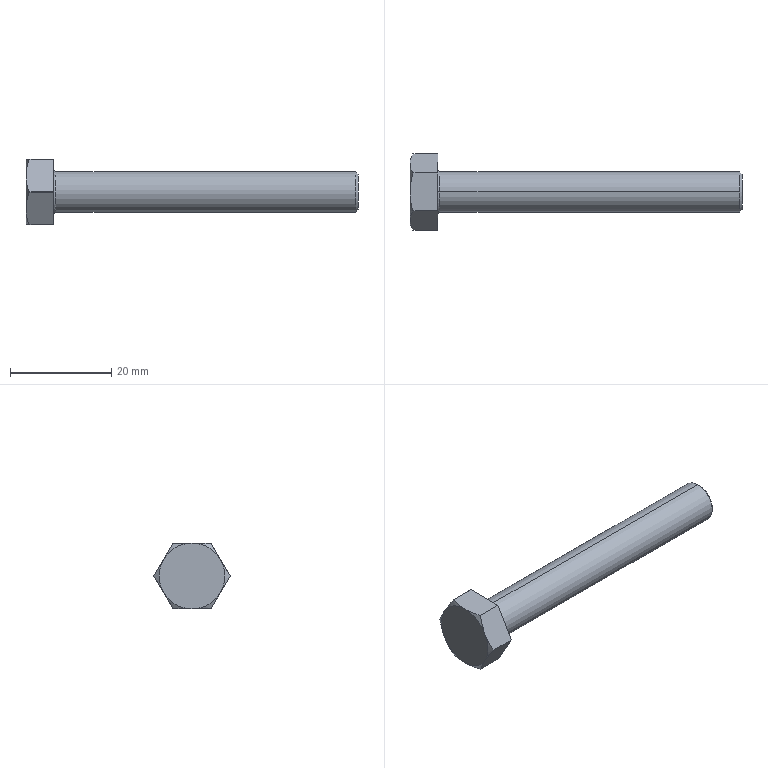Part | NX | features STRCB8-60 2 | 1 solid | 27 faces | box 65.5 x 15 x 13 mm | volume 3817 mm3 | plane 9 | cone 8 | cylinder 8 | torus 2 | commonest cylinder face diameters 15 x6 8 x2
STEP:
#1=CARTESIAN_POINT('',(145.215,66.,-9.5));
#2=VERTEX_POINT('',#1);
#3=CARTESIAN_POINT('',(145.215,60.371,-6.25));
#4=VERTEX_POINT('',#3);
#5=CARTESIAN_POINT('',(145.215,66.,-3.));
#6=DIRECTION('',(-1.,0.,0.));
#7=DIRECTION('',(0.,0.,-1.));
#8=AXIS2_PLACEMENT_3D('',#5,#6,#7);
#9=CIRCLE('',#8,6.5);
#10=EDGE_CURVE('',#2,#4,#9,.T.);
#11=ORIENTED_EDGE('',*,*,#10,.F.);
#12=CARTESIAN_POINT('',(145.793,62.258,-9.5));
#13=VERTEX_POINT('',#12);
#14=CARTESIAN_POINT('',(145.215,66.,-9.5));
#15=CARTESIAN_POINT('',(145.214,64.733,-9.5));
#16=CARTESIAN_POINT('',(145.442,63.474,-9.5));
#17=CARTESIAN_POINT('',(145.793,62.258,-9.5));
#18=B_SPLINE_CURVE_WITH_KNOTS('',3,(#14,#15,#16,#17),.UNSPECIFIED.,.F.,.F.,(4,4),(0.,1.),.UNSPECIFIED.);
#19=EDGE_CURVE('',#2,#13,#18,.T.);
#20=ORIENTED_EDGE('',*,*,#19,.T.);
#21=CARTESIAN_POINT('',(145.793,62.242,-9.49));
#22=VERTEX_POINT('',#21);
#23=CARTESIAN_POINT('',(145.793,66.,-3.));
#24=DIRECTION('',(-1.,0.,0.));
#25=DIRECTION('',(0.,-0.4989,-0.8667));
#26=AXIS2_PLACEMENT_3D('',#23,#24,#25);
#27=CIRCLE('',#26,7.5);
#28=EDGE_CURVE('',#13,#22,#27,.T.);
#29=ORIENTED_EDGE('',*,*,#28,.T.);
#30=CARTESIAN_POINT('',(145.793,62.242,-9.49));
#31=CARTESIAN_POINT('',(145.442,61.634,-8.437));
#32=CARTESIAN_POINT('',(145.214,61.004,-7.347));
#33=CARTESIAN_POINT('',(145.215,60.371,-6.25));
#34=B_SPLINE_CURVE_WITH_KNOTS('',3,(#30,#31,#32,#33),.UNSPECIFIED.,.F.,.F.,(4,4),(0.,1.),.UNSPECIFIED.);
#35=EDGE_CURVE('',#22,#4,#34,.T.);
#36=ORIENTED_EDGE('',*,*,#35,.T.);
#37=EDGE_LOOP('',(#11,#20,#29,#36));
#38=FACE_BOUND('',#37,.T.);
#39=CARTESIAN_POINT('',(145.174,66.,-3.));
#40=DIRECTION('',(1.,0.,0.));
#41=DIRECTION('',(0.,0.,1.));
#42=AXIS2_PLACEMENT_3D('',#39,#40,#41);
#43=CONICAL_SURFACE('',#42,6.428,1.047);
#44=ADVANCED_FACE('',(#38),#43,.T.);
#45=CARTESIAN_POINT('',(145.793,58.5,-3.01));
#46=VERTEX_POINT('',#45);
#47=CARTESIAN_POINT('',(145.793,58.5,-2.99));
#48=VERTEX_POINT('',#47);
#49=CARTESIAN_POINT('',(145.793,66.,-3.));
#50=DIRECTION('',(-1.,0.,0.));
#51=DIRECTION('',(0.,-1.,-0.001284));
#52=AXIS2_PLACEMENT_3D('',#49,#50,#51);
#53=CIRCLE('',#52,7.5);
#54=EDGE_CURVE('',#46,#48,#53,.T.);
#55=ORIENTED_EDGE('',*,*,#54,.T.);
#56=CARTESIAN_POINT('',(145.215,60.371,0.25));
#57=VERTEX_POINT('',#56);
#58=CARTESIAN_POINT('',(145.793,58.5,-2.99));
#59=CARTESIAN_POINT('',(145.442,59.108,-1.937));
#60=CARTESIAN_POINT('',(145.214,59.737,-0.847));
#61=CARTESIAN_POINT('',(145.215,60.371,0.25));
#62=B_SPLINE_CURVE_WITH_KNOTS('',3,(#58,#59,#60,#61),.UNSPECIFIED.,.F.,.F.,(4,4),(0.,1.),.UNSPECIFIED.);
#63=EDGE_CURVE('',#48,#57,#62,.T.);
#64=ORIENTED_EDGE('',*,*,#63,.T.);
#65=CARTESIAN_POINT('',(145.215,66.,-3.));
#66=DIRECTION('',(-1.,0.,0.));
#67=DIRECTION('',(0.,-0.866,-0.5));
#68=AXIS2_PLACEMENT_3D('',#65,#66,#67);
#69=CIRCLE('',#68,6.5);
#70=EDGE_CURVE('',#4,#57,#69,.T.);
#71=ORIENTED_EDGE('',*,*,#70,.F.);
#72=CARTESIAN_POINT('',(145.215,60.371,-6.25));
#73=CARTESIAN_POINT('',(145.214,59.737,-5.153));
#74=CARTESIAN_POINT('',(145.442,59.108,-4.063));
#75=CARTESIAN_POINT('',(145.793,58.5,-3.01));
#76=B_SPLINE_CURVE_WITH_KNOTS('',3,(#72,#73,#74,#75),.UNSPECIFIED.,.F.,.F.,(4,4),(0.,1.),.UNSPECIFIED.);
#77=EDGE_CURVE('',#4,#46,#76,.T.);
#78=ORIENTED_EDGE('',*,*,#77,.T.);
#79=EDGE_LOOP('',(#55,#64,#71,#78));
#80=FACE_BOUND('',#79,.T.);
#81=CARTESIAN_POINT('',(145.174,66.,-3.));
#82=DIRECTION('',(1.,0.,0.));
#83=DIRECTION('',(0.,0.,1.));
#84=AXIS2_PLACEMENT_3D('',#81,#82,#83);
#85=CONICAL_SURFACE('',#84,6.428,1.047);
#86=ADVANCED_FACE('',(#80),#85,.T.);
#87=CARTESIAN_POINT('',(145.215,66.,3.5));
#88=VERTEX_POINT('',#87);
#89=CARTESIAN_POINT('',(145.215,66.,-3.));
#90=DIRECTION('',(-1.,0.,0.));
#91=DIRECTION('',(0.,-0.866,0.5));
#92=AXIS2_PLACEMENT_3D('',#89,#90,#91);
#93=CIRCLE('',#92,6.5);
#94=EDGE_CURVE('',#57,#88,#93,.T.);
#95=ORIENTED_EDGE('',*,*,#94,.F.);
#96=CARTESIAN_POINT('',(145.793,62.242,3.49));
#97=VERTEX_POINT('',#96);
#98=CARTESIAN_POINT('',(145.215,60.371,0.25));
#99=CARTESIAN_POINT('',(145.214,61.004,1.347));
#100=CARTESIAN_POINT('',(145.442,61.634,2.437));
#101=CARTESIAN_POINT('',(145.793,62.242,3.49));
#102=B_SPLINE_CURVE_WITH_KNOTS('',3,(#98,#99,#100,#101),.UNSPECIFIED.,.F.,.F.,(4,4),(0.,1.),.UNSPECIFIED.);
#103=EDGE_CURVE('',#57,#97,#102,.T.);
#104=ORIENTED_EDGE('',*,*,#103,.T.);
#105=CARTESIAN_POINT('',(145.793,62.258,3.5));
#106=VERTEX_POINT('',#105);
#107=CARTESIAN_POINT('',(145.793,66.,-3.));
#108=DIRECTION('',(-1.,0.,0.));
#109=DIRECTION('',(0.,-0.5011,0.8654));
#110=AXIS2_PLACEMENT_3D('',#107,#108,#109);
#111=CIRCLE('',#110,7.5);
#112=EDGE_CURVE('',#97,#106,#111,.T.);
#113=ORIENTED_EDGE('',*,*,#112,.T.);
#114=CARTESIAN_POINT('',(145.793,62.258,3.5));
#115=CARTESIAN_POINT('',(145.442,63.474,3.5));
#116=CARTESIAN_POINT('',(145.214,64.733,3.5));
#117=CARTESIAN_POINT('',(145.215,66.,3.5));
#118=B_SPLINE_CURVE_WITH_KNOTS('',3,(#114,#115,#116,#117),.UNSPECIFIED.,.F.,.F.,(4,4),(0.,1.),.UNSPECIFIED.);
#119=EDGE_CURVE('',#106,#88,#118,.T.);
#120=ORIENTED_EDGE('',*,*,#119,.T.);
#121=EDGE_LOOP('',(#95,#104,#113,#120));
#122=FACE_BOUND('',#121,.T.);
#123=CARTESIAN_POINT('',(145.174,66.,-3.));
#124=DIRECTION('',(1.,0.,0.));
#125=DIRECTION('',(0.,0.,1.));
#126=AXIS2_PLACEMENT_3D('',#123,#124,#125);
#127=CONICAL_SURFACE('',#126,6.428,1.047);
#128=ADVANCED_FACE('',(#122),#127,.T.);
#129=CARTESIAN_POINT('',(145.793,73.5,-2.99));
#130=VERTEX_POINT('',#129);
#131=CARTESIAN_POINT('',(145.793,73.5,-3.01));
#132=VERTEX_POINT('',#131);
#133=CARTESIAN_POINT('',(145.793,66.,-3.));
#134=DIRECTION('',(-1.,0.,0.));
#135=DIRECTION('',(0.,1.,0.001284));
#136=AXIS2_PLACEMENT_3D('',#133,#134,#135);
#137=CIRCLE('',#136,7.5);
#138=EDGE_CURVE('',#130,#132,#137,.T.);
#139=ORIENTED_EDGE('',*,*,#138,.T.);
#140=CARTESIAN_POINT('',(145.215,71.629,-6.25));
#141=VERTEX_POINT('',#140);
#142=CARTESIAN_POINT('',(145.793,73.5,-3.01));
#143=CARTESIAN_POINT('',(145.442,72.892,-4.063));
#144=CARTESIAN_POINT('',(145.214,72.263,-5.153));
#145=CARTESIAN_POINT('',(145.215,71.629,-6.25));
#146=B_SPLINE_CURVE_WITH_KNOTS('',3,(#142,#143,#144,#145),.UNSPECIFIED.,.F.,.F.,(4,4),(0.,1.),.UNSPECIFIED.);
#147=EDGE_CURVE('',#132,#141,#146,.T.);
#148=ORIENTED_EDGE('',*,*,#147,.T.);
#149=CARTESIAN_POINT('',(145.215,71.629,0.25));
#150=VERTEX_POINT('',#149);
#151=CARTESIAN_POINT('',(145.215,66.,-3.));
#152=DIRECTION('',(-1.,0.,0.));
#153=DIRECTION('',(0.,0.866,0.5));
#154=AXIS2_PLACEMENT_3D('',#151,#152,#153);
#155=CIRCLE('',#154,6.5);
#156=EDGE_CURVE('',#150,#141,#155,.T.);
#157=ORIENTED_EDGE('',*,*,#156,.F.);
#158=CARTESIAN_POINT('',(145.215,71.629,0.25));
#159=CARTESIAN_POINT('',(145.214,72.263,-0.847));
#160=CARTESIAN_POINT('',(145.442,72.892,-1.937));
#161=CARTESIAN_POINT('',(145.793,73.5,-2.99));
#162=B_SPLINE_CURVE_WITH_KNOTS('',3,(#158,#159,#160,#161),.UNSPECIFIED.,.F.,.F.,(4,4),(0.,1.),.UNSPECIFIED.);
#163=EDGE_CURVE('',#150,#130,#162,.T.);
#164=ORIENTED_EDGE('',*,*,#163,.T.);
#165=EDGE_LOOP('',(#139,#148,#157,#164));
#166=FACE_BOUND('',#165,.T.);
#167=CARTESIAN_POINT('',(145.174,66.,-3.));
#168=DIRECTION('',(1.,0.,0.));
#169=DIRECTION('',(0.,0.,1.));
#170=AXIS2_PLACEMENT_3D('',#167,#168,#169);
#171=CONICAL_SURFACE('',#170,6.428,1.047);
#172=ADVANCED_FACE('',(#166),#171,.T.);
#173=CARTESIAN_POINT('',(145.215,66.,-3.));
#174=DIRECTION('',(-1.,0.,0.));
#175=DIRECTION('',(0.,0.866,-0.5));
#176=AXIS2_PLACEMENT_3D('',#173,#174,#175);
#177=CIRCLE('',#176,6.5);
#178=EDGE_CURVE('',#141,#2,#177,.T.);
#179=ORIENTED_EDGE('',*,*,#178,.F.);
#180=CARTESIAN_POINT('',(145.793,69.758,-9.49));
#181=VERTEX_POINT('',#180);
#182=CARTESIAN_POINT('',(145.215,71.629,-6.25));
#183=CARTESIAN_POINT('',(145.214,70.996,-7.347));
#184=CARTESIAN_POINT('',(145.442,70.366,-8.437));
#185=CARTESIAN_POINT('',(145.793,69.758,-9.49));
#186=B_SPLINE_CURVE_WITH_KNOTS('',3,(#182,#183,#184,#185),.UNSPECIFIED.,.F.,.F.,(4,4),(0.,1.),.UNSPECIFIED.);
#187=EDGE_CURVE('',#141,#181,#186,.T.);
#188=ORIENTED_EDGE('',*,*,#187,.T.);
#189=CARTESIAN_POINT('',(145.793,69.742,-9.5));
#190=VERTEX_POINT('',#189);
#191=CARTESIAN_POINT('',(145.793,66.,-3.));
#192=DIRECTION('',(-1.,0.,0.));
#193=DIRECTION('',(0.,0.5011,-0.8654));
#194=AXIS2_PLACEMENT_3D('',#191,#192,#193);
#195=CIRCLE('',#194,7.5);
#196=EDGE_CURVE('',#181,#190,#195,.T.);
#197=ORIENTED_EDGE('',*,*,#196,.T.);
#198=CARTESIAN_POINT('',(145.793,69.742,-9.5));
#199=CARTESIAN_POINT('',(145.442,68.526,-9.5));
#200=CARTESIAN_POINT('',(145.214,67.267,-9.5));
#201=CARTESIAN_POINT('',(145.215,66.,-9.5));
#202=B_SPLINE_CURVE_WITH_KNOTS('',3,(#198,#199,#200,#201),.UNSPECIFIED.,.F.,.F.,(4,4),(0.,1.),.UNSPECIFIED.);
#203=EDGE_CURVE('',#190,#2,#202,.T.);
#204=ORIENTED_EDGE('',*,*,#203,.T.);
#205=EDGE_LOOP('',(#179,#188,#197,#204));
#206=FACE_BOUND('',#205,.T.);
#207=CARTESIAN_POINT('',(145.174,66.,-3.));
#208=DIRECTION('',(1.,0.,0.));
#209=DIRECTION('',(0.,0.,1.));
#210=AXIS2_PLACEMENT_3D('',#207,#208,#209);
#211=CONICAL_SURFACE('',#210,6.428,1.047);
#212=ADVANCED_FACE('',(#206),#211,.T.);
#213=ORIENTED_EDGE('',*,*,#10,.T.);
#214=ORIENTED_EDGE('',*,*,#70,.T.);
#215=ORIENTED_EDGE('',*,*,#94,.T.);
#216=CARTESIAN_POINT('',(145.215,66.,-3.));
#217=DIRECTION('',(-1.,0.,0.));
#218=DIRECTION('',(0.,0.,1.));
#219=AXIS2_PLACEMENT_3D('',#216,#217,#218);
#220=CIRCLE('',#219,6.5);
#221=EDGE_CURVE('',#88,#150,#220,.T.);
#222=ORIENTED_EDGE('',*,*,#221,.T.);
#223=ORIENTED_EDGE('',*,*,#156,.T.);
#224=ORIENTED_EDGE('',*,*,#178,.T.);
#225=EDGE_LOOP('',(#213,#214,#215,#222,#223,#224));
#226=FACE_BOUND('',#225,.T.);
#227=CARTESIAN_POINT('',(145.215,62.75,-3.));
#228=DIRECTION('',(-1.,0.,0.));
#229=DIRECTION('',(0.,0.,-1.));
#230=AXIS2_PLACEMENT_3D('',#227,#228,#229);
#231=PLANE('',#230);
#232=ADVANCED_FACE('',(#226),#231,.T.);
#233=ORIENTED_EDGE('',*,*,#221,.F.);
#234=CARTESIAN_POINT('',(145.793,69.742,3.5));
#235=VERTEX_POINT('',#234);
#236=CARTESIAN_POINT('',(145.215,66.,3.5));
#237=CARTESIAN_POINT('',(145.214,67.267,3.5));
#238=CARTESIAN_POINT('',(145.442,68.526,3.5));
#239=CARTESIAN_POINT('',(145.793,69.742,3.5));
#240=B_SPLINE_CURVE_WITH_KNOTS('',3,(#236,#237,#238,#239),.UNSPECIFIED.,.F.,.F.,(4,4),(0.,1.),.UNSPECIFIED.);
#241=EDGE_CURVE('',#88,#235,#240,.T.);
#242=ORIENTED_EDGE('',*,*,#241,.T.);
#243=CARTESIAN_POINT('',(145.793,69.758,3.49));
#244=VERTEX_POINT('',#243);
#245=CARTESIAN_POINT('',(145.793,66.,-3.));
#246=DIRECTION('',(-1.,0.,0.));
#247=DIRECTION('',(0.,0.4989,0.8667));
#248=AXIS2_PLACEMENT_3D('',#245,#246,#247);
#249=CIRCLE('',#248,7.5);
#250=EDGE_CURVE('',#235,#244,#249,.T.);
#251=ORIENTED_EDGE('',*,*,#250,.T.);
#252=CARTESIAN_POINT('',(145.793,69.758,3.49));
#253=CARTESIAN_POINT('',(145.442,70.366,2.437));
#254=CARTESIAN_POINT('',(145.214,70.996,1.347));
#255=CARTESIAN_POINT('',(145.215,71.629,0.25));
#256=B_SPLINE_CURVE_WITH_KNOTS('',3,(#252,#253,#254,#255),.UNSPECIFIED.,.F.,.F.,(4,4),(0.,1.),.UNSPECIFIED.);
#257=EDGE_CURVE('',#244,#150,#256,.T.);
#258=ORIENTED_EDGE('',*,*,#257,.T.);
#259=EDGE_LOOP('',(#233,#242,#251,#258));
#260=FACE_BOUND('',#259,.T.);
#261=CARTESIAN_POINT('',(145.174,66.,-3.));
#262=DIRECTION('',(1.,0.,0.));
#263=DIRECTION('',(0.,0.,1.));
#264=AXIS2_PLACEMENT_3D('',#261,#262,#263);
#265=CONICAL_SURFACE('',#264,6.428,1.047);
#266=ADVANCED_FACE('',(#260),#265,.T.);
#267=ORIENTED_EDGE('',*,*,#250,.F.);
#268=CARTESIAN_POINT('',(150.715,69.742,3.5));
#269=VERTEX_POINT('',#268);
#270=CARTESIAN_POINT('',(145.793,69.742,3.5));
#271=DIRECTION('',(1.,0.,0.));
#272=VECTOR('',#271,1000.);
#273=LINE('',#270,#272);
#274=EDGE_CURVE('',#235,#269,#273,.T.);
#275=ORIENTED_EDGE('',*,*,#274,.T.);
#276=CARTESIAN_POINT('',(150.715,69.758,3.49));
#277=VERTEX_POINT('',#276);
#278=CARTESIAN_POINT('',(150.715,66.,-3.));
#279=DIRECTION('',(1.,0.,0.));
#280=DIRECTION('',(0.,0.5011,0.8654));
#281=AXIS2_PLACEMENT_3D('',#278,#279,#280);
#282=CIRCLE('',#281,7.5);
#283=EDGE_CURVE('',#277,#269,#282,.T.);
#284=ORIENTED_EDGE('',*,*,#283,.F.);
#285=CARTESIAN_POINT('',(150.715,69.758,3.49));
#286=DIRECTION('',(-1.,0.,0.));
#287=VECTOR('',#286,1000.);
#288=LINE('',#285,#287);
#289=EDGE_CURVE('',#277,#244,#288,.T.);
#290=ORIENTED_EDGE('',*,*,#289,.T.);
#291=EDGE_LOOP('',(#267,#275,#284,#290));
#292=FACE_BOUND('',#291,.T.);
#293=CARTESIAN_POINT('',(148.254,66.,-3.));
#294=DIRECTION('',(1.,0.,0.));
#295=DIRECTION('',(0.,0.,1.));
#296=AXIS2_PLACEMENT_3D('',#293,#294,#295);
#297=CYLINDRICAL_SURFACE('',#296,7.5);
#298=ADVANCED_FACE('',(#292),#297,.T.);
#299=CARTESIAN_POINT('',(150.715,73.5,-2.99));
#300=VERTEX_POINT('',#299);
#301=CARTESIAN_POINT('',(145.793,73.5,-2.99));
#302=DIRECTION('',(1.,0.,0.));
#303=VECTOR('',#302,1000.);
#304=LINE('',#301,#303);
#305=EDGE_CURVE('',#130,#300,#304,.T.);
#306=ORIENTED_EDGE('',*,*,#305,.F.);
#307=ORIENTED_EDGE('',*,*,#163,.F.);
#308=ORIENTED_EDGE('',*,*,#257,.F.);
#309=ORIENTED_EDGE('',*,*,#289,.F.);
#310=CARTESIAN_POINT('',(150.715,73.5,-2.99));
#311=DIRECTION('',(0.,-0.5,0.866));
#312=VECTOR('',#311,1000.);
#313=LINE('',#310,#312);
#314=EDGE_CURVE('',#300,#277,#313,.T.);
#315=ORIENTED_EDGE('',*,*,#314,.F.);
#316=EDGE_LOOP('',(#306,#307,#308,#309,#315));
#317=FACE_BOUND('',#316,.T.);
#318=CARTESIAN_POINT('',(150.715,69.753,3.5));
#319=DIRECTION('',(0.,-0.866,-0.5));
#320=DIRECTION('',(0.,0.5,-0.866));
#321=AXIS2_PLACEMENT_3D('',#318,#319,#320);
#322=PLANE('',#321);
#323=ADVANCED_FACE('',(#317),#322,.F.);
#324=CARTESIAN_POINT('',(150.715,73.5,-3.01));
#325=VERTEX_POINT('',#324);
#326=CARTESIAN_POINT('',(150.715,66.,-3.));
#327=DIRECTION('',(1.,0.,0.));
#328=DIRECTION('',(0.,1.,-0.001284));
#329=AXIS2_PLACEMENT_3D('',#326,#327,#328);
#330=CIRCLE('',#329,7.5);
#331=EDGE_CURVE('',#325,#300,#330,.T.);
#332=ORIENTED_EDGE('',*,*,#331,.F.);
#333=CARTESIAN_POINT('',(150.715,73.5,-3.01));
#334=DIRECTION('',(-1.,0.,0.));
#335=VECTOR('',#334,1000.);
#336=LINE('',#333,#335);
#337=EDGE_CURVE('',#325,#132,#336,.T.);
#338=ORIENTED_EDGE('',*,*,#337,.T.);
#339=ORIENTED_EDGE('',*,*,#138,.F.);
#340=ORIENTED_EDGE('',*,*,#305,.T.);
#341=EDGE_LOOP('',(#332,#338,#339,#340));
#342=FACE_BOUND('',#341,.T.);
#343=CARTESIAN_POINT('',(148.254,66.,-3.));
#344=DIRECTION('',(1.,0.,0.));
#345=DIRECTION('',(0.,0.,1.));
#346=AXIS2_PLACEMENT_3D('',#343,#344,#345);
#347=CYLINDRICAL_SURFACE('',#346,7.5);
#348=ADVANCED_FACE('',(#342),#347,.T.);
#349=CARTESIAN_POINT('',(150.715,69.758,-9.49));
#350=VERTEX_POINT('',#349);
#351=CARTESIAN_POINT('',(145.793,69.758,-9.49));
#352=DIRECTION('',(1.,0.,0.));
#353=VECTOR('',#352,1000.);
#354=LINE('',#351,#353);
#355=EDGE_CURVE('',#181,#350,#354,.T.);
#356=ORIENTED_EDGE('',*,*,#355,.F.);
#357=ORIENTED_EDGE('',*,*,#187,.F.);
#358=ORIENTED_EDGE('',*,*,#147,.F.);
#359=ORIENTED_EDGE('',*,*,#337,.F.);
#360=CARTESIAN_POINT('',(150.715,69.758,-9.49));
#361=DIRECTION('',(0.,0.5,0.866));
#362=VECTOR('',#361,1000.);
#363=LINE('',#360,#362);
#364=EDGE_CURVE('',#350,#325,#363,.T.);
#365=ORIENTED_EDGE('',*,*,#364,.F.);
#366=EDGE_LOOP('',(#356,#357,#358,#359,#365));
#367=FACE_BOUND('',#366,.T.);
#368=CARTESIAN_POINT('',(150.715,73.506,-3.));
#369=DIRECTION('',(0.,-0.866,0.5));
#370=DIRECTION('',(0.,-0.5,-0.866));
#371=AXIS2_PLACEMENT_3D('',#368,#369,#370);
#372=PLANE('',#371);
#373=ADVANCED_FACE('',(#367),#372,.F.);
#374=ORIENTED_EDGE('',*,*,#196,.F.);
#375=ORIENTED_EDGE('',*,*,#355,.T.);
#376=CARTESIAN_POINT('',(150.715,69.742,-9.5));
#377=VERTEX_POINT('',#376);
#378=CARTESIAN_POINT('',(150.715,66.,-3.));
#379=DIRECTION('',(1.,0.,0.));
#380=DIRECTION('',(0.,0.4989,-0.8667));
#381=AXIS2_PLACEMENT_3D('',#378,#379,#380);
#382=CIRCLE('',#381,7.5);
#383=EDGE_CURVE('',#377,#350,#382,.T.);
#384=ORIENTED_EDGE('',*,*,#383,.F.);
#385=CARTESIAN_POINT('',(150.715,69.742,-9.5));
#386=DIRECTION('',(-1.,0.,0.));
#387=VECTOR('',#386,1000.);
#388=LINE('',#385,#387);
#389=EDGE_CURVE('',#377,#190,#388,.T.);
#390=ORIENTED_EDGE('',*,*,#389,.T.);
#391=EDGE_LOOP('',(#374,#375,#384,#390));
#392=FACE_BOUND('',#391,.T.);
#393=CARTESIAN_POINT('',(148.254,66.,-3.));
#394=DIRECTION('',(1.,0.,0.));
#395=DIRECTION('',(0.,0.,1.));
#396=AXIS2_PLACEMENT_3D('',#393,#394,#395);
#397=CYLINDRICAL_SURFACE('',#396,7.5);
#398=ADVANCED_FACE('',(#392),#397,.T.);
#399=CARTESIAN_POINT('',(150.715,62.258,-9.5));
#400=VERTEX_POINT('',#399);
#401=CARTESIAN_POINT('',(145.793,62.258,-9.5));
#402=DIRECTION('',(1.,0.,0.));
#403=VECTOR('',#402,1000.);
#404=LINE('',#401,#403);
#405=EDGE_CURVE('',#13,#400,#404,.T.);
#406=ORIENTED_EDGE('',*,*,#405,.F.);
#407=ORIENTED_EDGE('',*,*,#19,.F.);
#408=ORIENTED_EDGE('',*,*,#203,.F.);
#409=ORIENTED_EDGE('',*,*,#389,.F.);
#410=CARTESIAN_POINT('',(150.715,69.742,-9.5));
#411=DIRECTION('',(0.,-1.,0.));
#412=VECTOR('',#411,1000.);
#413=LINE('',#410,#412);
#414=EDGE_CURVE('',#377,#400,#413,.T.);
#415=ORIENTED_EDGE('',*,*,#414,.T.);
#416=EDGE_LOOP('',(#406,#407,#408,#409,#415));
#417=FACE_BOUND('',#416,.T.);
#418=CARTESIAN_POINT('',(150.715,69.753,-9.5));
#419=DIRECTION('',(0.,0.,1.));
#420=DIRECTION('',(-1.,0.,0.));
#421=AXIS2_PLACEMENT_3D('',#418,#419,#420);
#422=PLANE('',#421);
#423=ADVANCED_FACE('',(#417),#422,.F.);
#424=ORIENTED_EDGE('',*,*,#28,.F.);
#425=ORIENTED_EDGE('',*,*,#405,.T.);
#426=CARTESIAN_POINT('',(150.715,62.242,-9.49));
#427=VERTEX_POINT('',#426);
#428=CARTESIAN_POINT('',(150.715,66.,-3.));
#429=DIRECTION('',(1.,0.,0.));
#430=DIRECTION('',(0.,-0.5011,-0.8654));
#431=AXIS2_PLACEMENT_3D('',#428,#429,#430);
#432=CIRCLE('',#431,7.5);
#433=EDGE_CURVE('',#427,#400,#432,.T.);
#434=ORIENTED_EDGE('',*,*,#433,.F.);
#435=CARTESIAN_POINT('',(150.715,62.242,-9.49));
#436=DIRECTION('',(-1.,0.,0.));
#437=VECTOR('',#436,1000.);
#438=LINE('',#435,#437);
#439=EDGE_CURVE('',#427,#22,#438,.T.);
#440=ORIENTED_EDGE('',*,*,#439,.T.);
#441=EDGE_LOOP('',(#424,#425,#434,#440));
#442=FACE_BOUND('',#441,.T.);
#443=CARTESIAN_POINT('',(148.254,66.,-3.));
#444=DIRECTION('',(1.,0.,0.));
#445=DIRECTION('',(0.,0.,1.));
#446=AXIS2_PLACEMENT_3D('',#443,#444,#445);
#447=CYLINDRICAL_SURFACE('',#446,7.5);
#448=ADVANCED_FACE('',(#442),#447,.T.);
#449=CARTESIAN_POINT('',(150.715,58.5,-3.01));
#450=VERTEX_POINT('',#449);
#451=CARTESIAN_POINT('',(145.793,58.5,-3.01));
#452=DIRECTION('',(1.,0.,0.));
#453=VECTOR('',#452,1000.);
#454=LINE('',#451,#453);
#455=EDGE_CURVE('',#46,#450,#454,.T.);
#456=ORIENTED_EDGE('',*,*,#455,.F.);
#457=ORIENTED_EDGE('',*,*,#77,.F.);
#458=ORIENTED_EDGE('',*,*,#35,.F.);
#459=ORIENTED_EDGE('',*,*,#439,.F.);
#460=CARTESIAN_POINT('',(150.715,58.5,-3.01));
#461=DIRECTION('',(0.,0.5,-0.866));
#462=VECTOR('',#461,1000.);
#463=LINE('',#460,#462);
#464=EDGE_CURVE('',#450,#427,#463,.T.);
#465=ORIENTED_EDGE('',*,*,#464,.F.);
#466=EDGE_LOOP('',(#456,#457,#458,#459,#465));
#467=FACE_BOUND('',#466,.T.);
#468=CARTESIAN_POINT('',(150.715,62.247,-9.5));
#469=DIRECTION('',(0.,0.866,0.5));
#470=DIRECTION('',(0.,-0.5,0.866));
#471=AXIS2_PLACEMENT_3D('',#468,#469,#470);
#472=PLANE('',#471);
#473=ADVANCED_FACE('',(#467),#472,.F.);
#474=CARTESIAN_POINT('',(150.715,58.5,-2.99));
#475=VERTEX_POINT('',#474);
#476=CARTESIAN_POINT('',(150.715,66.,-3.));
#477=DIRECTION('',(1.,0.,0.));
#478=DIRECTION('',(0.,-1.,0.001284));
#479=AXIS2_PLACEMENT_3D('',#476,#477,#478);
#480=CIRCLE('',#479,7.5);
#481=EDGE_CURVE('',#475,#450,#480,.T.);
#482=ORIENTED_EDGE('',*,*,#481,.F.);
#483=CARTESIAN_POINT('',(150.715,58.5,-2.99));
#484=DIRECTION('',(-1.,0.,0.));
#485=VECTOR('',#484,1000.);
#486=LINE('',#483,#485);
#487=EDGE_CURVE('',#475,#48,#486,.T.);
#488=ORIENTED_EDGE('',*,*,#487,.T.);
#489=ORIENTED_EDGE('',*,*,#54,.F.);
#490=ORIENTED_EDGE('',*,*,#455,.T.);
#491=EDGE_LOOP('',(#482,#488,#489,#490));
#492=FACE_BOUND('',#491,.T.);
#493=CARTESIAN_POINT('',(148.254,66.,-3.));
#494=DIRECTION('',(1.,0.,0.));
#495=DIRECTION('',(0.,0.,1.));
#496=AXIS2_PLACEMENT_3D('',#493,#494,#495);
#497=CYLINDRICAL_SURFACE('',#496,7.5);
#498=ADVANCED_FACE('',(#492),#497,.T.);
#499=CARTESIAN_POINT('',(150.715,62.242,3.49));
#500=VERTEX_POINT('',#499);
#501=CARTESIAN_POINT('',(145.793,62.242,3.49));
#502=DIRECTION('',(1.,0.,0.));
#503=VECTOR('',#502,1000.);
#504=LINE('',#501,#503);
#505=EDGE_CURVE('',#97,#500,#504,.T.);
#506=ORIENTED_EDGE('',*,*,#505,.F.);
#507=ORIENTED_EDGE('',*,*,#103,.F.);
#508=ORIENTED_EDGE('',*,*,#63,.F.);
#509=ORIENTED_EDGE('',*,*,#487,.F.);
#510=CARTESIAN_POINT('',(150.715,62.242,3.49));
#511=DIRECTION('',(0.,-0.5,-0.866));
#512=VECTOR('',#511,1000.);
#513=LINE('',#510,#512);
#514=EDGE_CURVE('',#500,#475,#513,.T.);
#515=ORIENTED_EDGE('',*,*,#514,.F.);
#516=EDGE_LOOP('',(#506,#507,#508,#509,#515));
#517=FACE_BOUND('',#516,.T.);
#518=CARTESIAN_POINT('',(150.715,58.494,-3.));
#519=DIRECTION('',(0.,0.866,-0.5));
#520=DIRECTION('',(0.,0.5,0.866));
#521=AXIS2_PLACEMENT_3D('',#518,#519,#520);
#522=PLANE('',#521);
#523=ADVANCED_FACE('',(#517),#522,.F.);
#524=ORIENTED_EDGE('',*,*,#112,.F.);
#525=ORIENTED_EDGE('',*,*,#505,.T.);
#526=CARTESIAN_POINT('',(150.715,62.258,3.5));
#527=VERTEX_POINT('',#526);
#528=CARTESIAN_POINT('',(150.715,66.,-3.));
#529=DIRECTION('',(1.,0.,0.));
#530=DIRECTION('',(0.,-0.4989,0.8667));
#531=AXIS2_PLACEMENT_3D('',#528,#529,#530);
#532=CIRCLE('',#531,7.5);
#533=EDGE_CURVE('',#527,#500,#532,.T.);
#534=ORIENTED_EDGE('',*,*,#533,.F.);
#535=CARTESIAN_POINT('',(150.715,62.258,3.5));
#536=DIRECTION('',(-1.,0.,0.));
#537=VECTOR('',#536,1000.);
#538=LINE('',#535,#537);
#539=EDGE_CURVE('',#527,#106,#538,.T.);
#540=ORIENTED_EDGE('',*,*,#539,.T.);
#541=EDGE_LOOP('',(#524,#525,#534,#540));
#542=FACE_BOUND('',#541,.T.);
#543=CARTESIAN_POINT('',(148.254,66.,-3.));
#544=DIRECTION('',(1.,0.,0.));
#545=DIRECTION('',(0.,0.,1.));
#546=AXIS2_PLACEMENT_3D('',#543,#544,#545);
#547=CYLINDRICAL_SURFACE('',#546,7.5);
#548=ADVANCED_FACE('',(#542),#547,.T.);
#549=ORIENTED_EDGE('',*,*,#274,.F.);
#550=ORIENTED_EDGE('',*,*,#241,.F.);
#551=ORIENTED_EDGE('',*,*,#119,.F.);
#552=ORIENTED_EDGE('',*,*,#539,.F.);
#553=CARTESIAN_POINT('',(150.715,62.258,3.5));
#554=DIRECTION('',(0.,1.,0.));
#555=VECTOR('',#554,1000.);
#556=LINE('',#553,#555);
#557=EDGE_CURVE('',#527,#269,#556,.T.);
#558=ORIENTED_EDGE('',*,*,#557,.T.);
#559=EDGE_LOOP('',(#549,#550,#551,#552,#558));
#560=FACE_BOUND('',#559,.T.);
#561=CARTESIAN_POINT('',(150.715,62.247,3.5));
#562=DIRECTION('',(0.,0.,-1.));
#563=DIRECTION('',(1.,0.,0.));
#564=AXIS2_PLACEMENT_3D('',#561,#562,#563);
#565=PLANE('',#564);
#566=ADVANCED_FACE('',(#560),#565,.F.);
#567=CARTESIAN_POINT('',(150.715,66.,-7.4));
#568=VERTEX_POINT('',#567);
#569=CARTESIAN_POINT('',(150.715,61.6,-2.999));
#570=VERTEX_POINT('',#569);
#571=CARTESIAN_POINT('',(150.715,66.,-3.));
#572=DIRECTION('',(-1.,0.,0.));
#573=DIRECTION('',(0.,-0.0002296,-1.));
#574=AXIS2_PLACEMENT_3D('',#571,#572,#573);
#575=CIRCLE('',#574,4.4);
#576=EDGE_CURVE('',#568,#570,#575,.T.);
#577=ORIENTED_EDGE('',*,*,#576,.T.);
#578=CARTESIAN_POINT('',(150.715,66.,1.4));
#579=VERTEX_POINT('',#578);
#580=CARTESIAN_POINT('',(150.715,66.,-3.));
#581=DIRECTION('',(-1.,0.,0.));
#582=DIRECTION('',(0.,-1.,0.0002618));
#583=AXIS2_PLACEMENT_3D('',#580,#581,#582);
#584=CIRCLE('',#583,4.4);
#585=EDGE_CURVE('',#570,#579,#584,.T.);
#586=ORIENTED_EDGE('',*,*,#585,.T.);
#587=CARTESIAN_POINT('',(150.715,66.,-3.));
#588=DIRECTION('',(-1.,0.,0.));
#589=DIRECTION('',(0.,0.0001052,1.));
#590=AXIS2_PLACEMENT_3D('',#587,#588,#589);
#591=CIRCLE('',#590,4.4);
#592=EDGE_CURVE('',#579,#568,#591,.T.);
#593=ORIENTED_EDGE('',*,*,#592,.T.);
#594=EDGE_LOOP('',(#577,#586,#593));
#595=FACE_BOUND('',#594,.T.);
#596=ORIENTED_EDGE('',*,*,#533,.T.);
#597=ORIENTED_EDGE('',*,*,#514,.T.);
#598=ORIENTED_EDGE('',*,*,#481,.T.);
#599=ORIENTED_EDGE('',*,*,#464,.T.);
#600=ORIENTED_EDGE('',*,*,#433,.T.);
#601=ORIENTED_EDGE('',*,*,#414,.F.);
#602=ORIENTED_EDGE('',*,*,#383,.T.);
#603=ORIENTED_EDGE('',*,*,#364,.T.);
#604=ORIENTED_EDGE('',*,*,#331,.T.);
#605=ORIENTED_EDGE('',*,*,#314,.T.);
#606=ORIENTED_EDGE('',*,*,#283,.T.);
#607=ORIENTED_EDGE('',*,*,#557,.F.);
#608=EDGE_LOOP('',(#596,#597,#598,#599,#600,#601,#602,#603,#604,#605,#606,#607));
#609=FACE_BOUND('',#608,.T.);
#610=CARTESIAN_POINT('',(150.715,60.05,-3.));
#611=DIRECTION('',(1.,0.,0.));
#612=DIRECTION('',(0.,0.,1.));
#613=AXIS2_PLACEMENT_3D('',#610,#611,#612);
#614=PLANE('',#613);
#615=ADVANCED_FACE('',(#595,#609),#614,.T.);
#616=CARTESIAN_POINT('',(151.115,66.,1.));
#617=VERTEX_POINT('',#616);
#618=CARTESIAN_POINT('',(151.115,66.,-7.));
#619=VERTEX_POINT('',#618);
#620=CARTESIAN_POINT('',(151.115,66.,-3.));
#621=DIRECTION('',(-1.,0.,0.));
#622=DIRECTION('',(0.,0.,1.));
#623=AXIS2_PLACEMENT_3D('',#620,#621,#622);
#624=CIRCLE('',#623,4.);
#625=EDGE_CURVE('',#617,#619,#624,.T.);
#626=ORIENTED_EDGE('',*,*,#625,.T.);
#627=CARTESIAN_POINT('',(151.115,66.,-7.4));
#628=DIRECTION('',(0.,1.,0.));
#629=DIRECTION('',(-1.,0.,0.));
#630=AXIS2_PLACEMENT_3D('',#627,#628,#629);
#631=CIRCLE('',#630,0.4);
#632=EDGE_CURVE('',#619,#568,#631,.F.);
#633=ORIENTED_EDGE('',*,*,#632,.T.);
#634=ORIENTED_EDGE('',*,*,#592,.F.);
#635=CARTESIAN_POINT('',(151.115,66.,1.4));
#636=DIRECTION('',(0.,-1.,0.));
#637=DIRECTION('',(-1.,0.,0.));
#638=AXIS2_PLACEMENT_3D('',#635,#636,#637);
#639=CIRCLE('',#638,0.4);
#640=EDGE_CURVE('',#579,#617,#639,.T.);
#641=ORIENTED_EDGE('',*,*,#640,.T.);
#642=EDGE_LOOP('',(#626,#633,#634,#641));
#643=FACE_BOUND('',#642,.T.);
#644=CARTESIAN_POINT('',(151.115,66.,-3.));
#645=DIRECTION('',(-1.,0.,0.));
#646=DIRECTION('',(0.,0.,1.));
#647=AXIS2_PLACEMENT_3D('',#644,#645,#646);
#648=TOROIDAL_SURFACE('',#647,4.4,0.4);
#649=ADVANCED_FACE('',(#643),#648,.F.);
#650=CARTESIAN_POINT('',(210.715,66.,-6.54));
#651=VERTEX_POINT('',#650);
#652=CARTESIAN_POINT('',(210.715,66.,0.54));
#653=VERTEX_POINT('',#652);
#654=CARTESIAN_POINT('',(210.715,66.,-3.));
#655=DIRECTION('',(1.,0.,0.));
#656=DIRECTION('',(0.,0.,-1.));
#657=AXIS2_PLACEMENT_3D('',#654,#655,#656);
#658=CIRCLE('',#657,3.54);
#659=EDGE_CURVE('',#651,#653,#658,.T.);
#660=ORIENTED_EDGE('',*,*,#659,.T.);
#661=CARTESIAN_POINT('',(210.715,66.,-3.));
#662=DIRECTION('',(1.,0.,0.));
#663=DIRECTION('',(0.,0.,1.));
#664=AXIS2_PLACEMENT_3D('',#661,#662,#663);
#665=CIRCLE('',#664,3.54);
#666=EDGE_CURVE('',#653,#651,#665,.T.);
#667=ORIENTED_EDGE('',*,*,#666,.T.);
#668=EDGE_LOOP('',(#660,#667));
#669=FACE_BOUND('',#668,.T.);
#670=CARTESIAN_POINT('',(210.715,64.23,-3.));
#671=DIRECTION('',(1.,0.,0.));
#672=DIRECTION('',(0.,0.,1.));
#673=AXIS2_PLACEMENT_3D('',#670,#671,#672);
#674=PLANE('',#673);
#675=ADVANCED_FACE('',(#669),#674,.T.);
#676=CARTESIAN_POINT('',(210.255,66.,1.));
#677=VERTEX_POINT('',#676);
#678=CARTESIAN_POINT('',(210.255,66.,1.));
#679=DIRECTION('',(0.7071,0.,-0.7071));
#680=VECTOR('',#679,1000.);
#681=LINE('',#678,#680);
#682=EDGE_CURVE('',#677,#653,#681,.T.);
#683=ORIENTED_EDGE('',*,*,#682,.F.);
#684=CARTESIAN_POINT('',(210.255,66.,-7.));
#685=VERTEX_POINT('',#684);
#686=CARTESIAN_POINT('',(210.255,66.,-3.));
#687=DIRECTION('',(1.,0.,0.));
#688=DIRECTION('',(0.,0.,1.));
#689=AXIS2_PLACEMENT_3D('',#686,#687,#688);
#690=CIRCLE('',#689,4.);
#691=EDGE_CURVE('',#677,#685,#690,.T.);
#692=ORIENTED_EDGE('',*,*,#691,.T.);
#693=CARTESIAN_POINT('',(210.255,66.,-7.));
#694=DIRECTION('',(0.7071,0.,0.7071));
#695=VECTOR('',#694,1000.);
#696=LINE('',#693,#695);
#697=EDGE_CURVE('',#651,#685,#696,.F.);
#698=ORIENTED_EDGE('',*,*,#697,.F.);
#699=ORIENTED_EDGE('',*,*,#666,.F.);
#700=EDGE_LOOP('',(#683,#692,#698,#699));
#701=FACE_BOUND('',#700,.T.);
#702=CARTESIAN_POINT('',(210.774,66.,-3.));
#703=DIRECTION('',(-1.,0.,0.));
#704=DIRECTION('',(0.,0.,-1.));
#705=AXIS2_PLACEMENT_3D('',#702,#703,#704);
#706=CONICAL_SURFACE('',#705,3.482,0.7854);
#707=ADVANCED_FACE('',(#701),#706,.T.);
#708=ORIENTED_EDGE('',*,*,#659,.F.);
#709=ORIENTED_EDGE('',*,*,#697,.T.);
#710=CARTESIAN_POINT('',(210.255,66.,-3.));
#711=DIRECTION('',(1.,0.,0.));
#712=DIRECTION('',(0.,0.,-1.));
#713=AXIS2_PLACEMENT_3D('',#710,#711,#712);
#714=CIRCLE('',#713,4.);
#715=EDGE_CURVE('',#685,#677,#714,.T.);
#716=ORIENTED_EDGE('',*,*,#715,.T.);
#717=ORIENTED_EDGE('',*,*,#682,.T.);
#718=EDGE_LOOP('',(#708,#709,#716,#717));
#719=FACE_BOUND('',#718,.T.);
#720=CARTESIAN_POINT('',(210.774,66.,-3.));
#721=DIRECTION('',(-1.,0.,0.));
#722=DIRECTION('',(0.,0.,-1.));
#723=AXIS2_PLACEMENT_3D('',#720,#721,#722);
#724=CONICAL_SURFACE('',#723,3.482,0.7854);
#725=ADVANCED_FACE('',(#719),#724,.T.);
#726=ORIENTED_EDGE('',*,*,#625,.F.);
#727=CARTESIAN_POINT('',(210.255,66.,1.));
#728=DIRECTION('',(-1.,0.,0.));
#729=VECTOR('',#728,1000.);
#730=LINE('',#727,#729);
#731=EDGE_CURVE('',#617,#677,#730,.F.);
#732=ORIENTED_EDGE('',*,*,#731,.T.);
#733=ORIENTED_EDGE('',*,*,#715,.F.);
#734=CARTESIAN_POINT('',(210.255,66.,-7.));
#735=DIRECTION('',(-1.,0.,0.));
#736=VECTOR('',#735,1000.);
#737=LINE('',#734,#736);
#738=EDGE_CURVE('',#685,#619,#737,.T.);
#739=ORIENTED_EDGE('',*,*,#738,.T.);
#740=EDGE_LOOP('',(#726,#732,#733,#739));
#741=FACE_BOUND('',#740,.T.);
#742=CARTESIAN_POINT('',(180.685,66.,-3.));
#743=DIRECTION('',(1.,0.,0.));
#744=DIRECTION('',(0.,0.,1.));
#745=AXIS2_PLACEMENT_3D('',#742,#743,#744);
#746=CYLINDRICAL_SURFACE('',#745,4.);
#747=ADVANCED_FACE('',(#741),#746,.T.);
#748=ORIENTED_EDGE('',*,*,#738,.F.);
#749=ORIENTED_EDGE('',*,*,#691,.F.);
#750=ORIENTED_EDGE('',*,*,#731,.F.);
#751=CARTESIAN_POINT('',(151.115,66.,-3.));
#752=DIRECTION('',(-1.,0.,0.));
#753=DIRECTION('',(0.,0.,-1.));
#754=AXIS2_PLACEMENT_3D('',#751,#752,#753);
#755=CIRCLE('',#754,4.);
#756=EDGE_CURVE('',#619,#617,#755,.T.);
#757=ORIENTED_EDGE('',*,*,#756,.F.);
#758=EDGE_LOOP('',(#748,#749,#750,#757));
#759=FACE_BOUND('',#758,.T.);
#760=CARTESIAN_POINT('',(180.685,66.,-3.));
#761=DIRECTION('',(1.,0.,0.));
#762=DIRECTION('',(0.,0.,1.));
#763=AXIS2_PLACEMENT_3D('',#760,#761,#762);
#764=CYLINDRICAL_SURFACE('',#763,4.);
#765=ADVANCED_FACE('',(#759),#764,.T.);
#766=ORIENTED_EDGE('',*,*,#640,.F.);
#767=ORIENTED_EDGE('',*,*,#585,.F.);
#768=ORIENTED_EDGE('',*,*,#576,.F.);
#769=ORIENTED_EDGE('',*,*,#632,.F.);
#770=ORIENTED_EDGE('',*,*,#756,.T.);
#771=EDGE_LOOP('',(#766,#767,#768,#769,#770));
#772=FACE_BOUND('',#771,.T.);
#773=CARTESIAN_POINT('',(151.115,66.,-3.));
#774=DIRECTION('',(-1.,0.,0.));
#775=DIRECTION('',(0.,0.,-1.));
#776=AXIS2_PLACEMENT_3D('',#773,#774,#775);
#777=TOROIDAL_SURFACE('',#776,4.4,0.4);
#778=ADVANCED_FACE('',(#772),#777,.F.);
#779=CLOSED_SHELL('',(#44,#86,#128,#172,#212,#232,#266,#298,#323,#348,#373,#398,#423,#448,#473,#498,#523,#548,#566,#615,#649,#675,#707,#725,#747,#765,#778));
#780=MANIFOLD_SOLID_BREP('',#779);
#781=(LENGTH_UNIT()NAMED_UNIT(*)SI_UNIT(.MILLI.,.METRE.));
#782=UNCERTAINTY_MEASURE_WITH_UNIT(LENGTH_MEASURE(0.0508),#781,'','');
#783=(NAMED_UNIT(*)PLANE_ANGLE_UNIT()SI_UNIT($,.RADIAN.));
#784=(NAMED_UNIT(*)SI_UNIT($,.STERADIAN.)SOLID_ANGLE_UNIT());
#785=(GEOMETRIC_REPRESENTATION_CONTEXT(3)GLOBAL_UNCERTAINTY_ASSIGNED_CONTEXT((#782))GLOBAL_UNIT_ASSIGNED_CONTEXT((#781,#783,#784))REPRESENTATION_CONTEXT('',''));
#786=ADVANCED_BREP_SHAPE_REPRESENTATION('',(#780),#785);